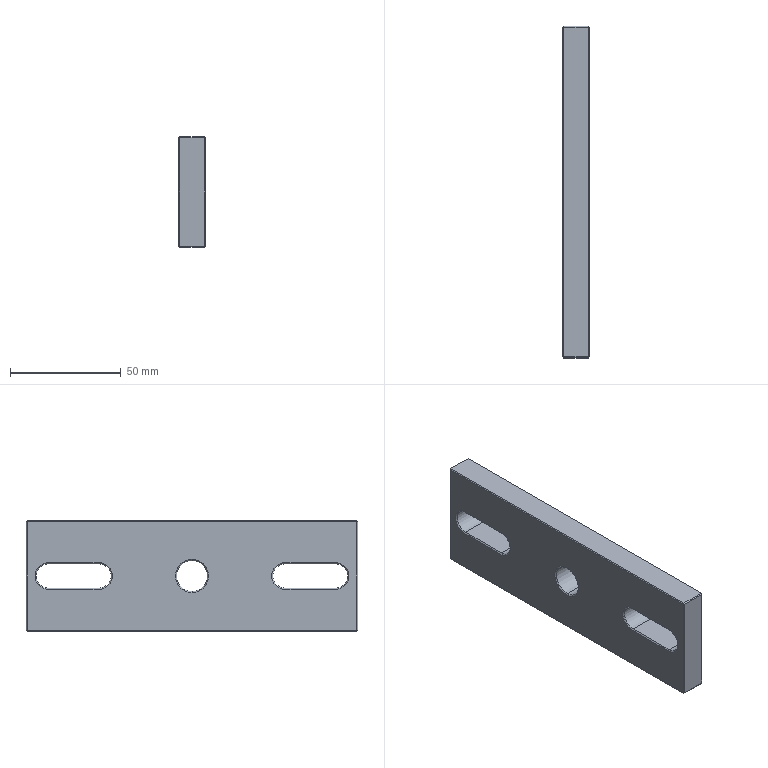Part | SolidWorks | features BaseBody 1 | 1 solid | 56 faces | box 12 x 150 x 50 mm | volume 79643 mm3 | plane 38 | cone 12 | cylinder 6 | commonest cylinder face diameters 11 x4 14 x2
STEP:
#1=CARTESIAN_POINT('',(-36.5,279.,-7.));
#2=VERTEX_POINT('',#1);
#3=CARTESIAN_POINT('',(-36.5,279.,7.));
#4=VERTEX_POINT('',#3);
#5=CARTESIAN_POINT('',(-36.5,279.,0.));
#6=DIRECTION('',(-1.,0.,0.));
#7=DIRECTION('',(0.,0.,1.));
#8=AXIS2_PLACEMENT_3D('',#5,#6,#7);
#9=CIRCLE('',#8,7.);
#10=EDGE_CURVE('',#2,#4,#9,.T.);
#11=ORIENTED_EDGE('',*,*,#10,.F.);
#12=CARTESIAN_POINT('',(-37.,279.,-7.5));
#13=VERTEX_POINT('',#12);
#14=CARTESIAN_POINT('',(-37.,279.,-7.5));
#15=DIRECTION('',(-0.7071,0.,-0.7071));
#16=VECTOR('',#15,1000.);
#17=LINE('',#14,#16);
#18=EDGE_CURVE('',#2,#13,#17,.T.);
#19=ORIENTED_EDGE('',*,*,#18,.T.);
#20=CARTESIAN_POINT('',(-37.,279.,7.5));
#21=VERTEX_POINT('',#20);
#22=CARTESIAN_POINT('',(-37.,279.,0.));
#23=DIRECTION('',(1.,0.,0.));
#24=DIRECTION('',(0.,0.,1.));
#25=AXIS2_PLACEMENT_3D('',#22,#23,#24);
#26=CIRCLE('',#25,7.5);
#27=EDGE_CURVE('',#21,#13,#26,.T.);
#28=ORIENTED_EDGE('',*,*,#27,.F.);
#29=CARTESIAN_POINT('',(-37.,279.,7.5));
#30=DIRECTION('',(-0.7071,0.,0.7071));
#31=VECTOR('',#30,1000.);
#32=LINE('',#29,#31);
#33=EDGE_CURVE('',#4,#21,#32,.T.);
#34=ORIENTED_EDGE('',*,*,#33,.F.);
#35=EDGE_LOOP('',(#11,#19,#28,#34));
#36=FACE_OUTER_BOUND('',#35,.T.);
#37=CARTESIAN_POINT('',(-37.,279.,0.));
#38=DIRECTION('',(-1.,0.,0.));
#39=DIRECTION('',(0.,0.,1.));
#40=AXIS2_PLACEMENT_3D('',#37,#38,#39);
#41=CONICAL_SURFACE('',#40,7.5,0.7854);
#42=ADVANCED_FACE('',(#36),#41,.F.);
#43=CARTESIAN_POINT('',(-25.5,279.,7.));
#44=VERTEX_POINT('',#43);
#45=CARTESIAN_POINT('',(-25.5,279.,-7.));
#46=VERTEX_POINT('',#45);
#47=CARTESIAN_POINT('',(-25.5,279.,0.));
#48=DIRECTION('',(1.,0.,0.));
#49=DIRECTION('',(0.,0.,1.));
#50=AXIS2_PLACEMENT_3D('',#47,#48,#49);
#51=CIRCLE('',#50,7.);
#52=EDGE_CURVE('',#44,#46,#51,.T.);
#53=ORIENTED_EDGE('',*,*,#52,.F.);
#54=CARTESIAN_POINT('',(-25.,279.,7.5));
#55=VERTEX_POINT('',#54);
#56=CARTESIAN_POINT('',(-25.5,279.,7.));
#57=DIRECTION('',(0.7071,0.,0.7071));
#58=VECTOR('',#57,1000.);
#59=LINE('',#56,#58);
#60=EDGE_CURVE('',#44,#55,#59,.T.);
#61=ORIENTED_EDGE('',*,*,#60,.T.);
#62=CARTESIAN_POINT('',(-25.,279.,-7.5));
#63=VERTEX_POINT('',#62);
#64=CARTESIAN_POINT('',(-25.,279.,0.));
#65=DIRECTION('',(-1.,0.,0.));
#66=DIRECTION('',(0.,0.,1.));
#67=AXIS2_PLACEMENT_3D('',#64,#65,#66);
#68=CIRCLE('',#67,7.5);
#69=EDGE_CURVE('',#63,#55,#68,.T.);
#70=ORIENTED_EDGE('',*,*,#69,.F.);
#71=CARTESIAN_POINT('',(-25.5,279.,-7.));
#72=DIRECTION('',(0.7071,0.,-0.7071));
#73=VECTOR('',#72,1000.);
#74=LINE('',#71,#73);
#75=EDGE_CURVE('',#46,#63,#74,.T.);
#76=ORIENTED_EDGE('',*,*,#75,.F.);
#77=EDGE_LOOP('',(#53,#61,#70,#76));
#78=FACE_OUTER_BOUND('',#77,.T.);
#79=CARTESIAN_POINT('',(-25.5,279.,0.));
#80=DIRECTION('',(1.,0.,0.));
#81=DIRECTION('',(0.,0.,-1.));
#82=AXIS2_PLACEMENT_3D('',#79,#80,#81);
#83=CONICAL_SURFACE('',#82,7.,0.7854);
#84=ADVANCED_FACE('',(#78),#83,.F.);
#85=ORIENTED_EDGE('',*,*,#10,.T.);
#86=CARTESIAN_POINT('',(-25.,279.,7.));
#87=DIRECTION('',(1.,0.,0.));
#88=VECTOR('',#87,1000.);
#89=LINE('',#86,#88);
#90=EDGE_CURVE('',#4,#44,#89,.T.);
#91=ORIENTED_EDGE('',*,*,#90,.T.);
#92=ORIENTED_EDGE('',*,*,#52,.T.);
#93=CARTESIAN_POINT('',(-25.,279.,-7.));
#94=DIRECTION('',(1.,0.,0.));
#95=VECTOR('',#94,1000.);
#96=LINE('',#93,#95);
#97=EDGE_CURVE('',#2,#46,#96,.T.);
#98=ORIENTED_EDGE('',*,*,#97,.F.);
#99=EDGE_LOOP('',(#85,#91,#92,#98));
#100=FACE_OUTER_BOUND('',#99,.T.);
#101=CARTESIAN_POINT('',(-25.,279.,0.));
#102=DIRECTION('',(1.,0.,0.));
#103=DIRECTION('',(0.,0.,-1.));
#104=AXIS2_PLACEMENT_3D('',#101,#102,#103);
#105=CYLINDRICAL_SURFACE('',#104,7.);
#106=ADVANCED_FACE('',(#100),#105,.F.);
#107=CARTESIAN_POINT('',(-36.5,214.,-5.5));
#108=VERTEX_POINT('',#107);
#109=CARTESIAN_POINT('',(-37.,214.,-6.));
#110=VERTEX_POINT('',#109);
#111=CARTESIAN_POINT('',(-36.5,214.,-5.5));
#112=DIRECTION('',(-0.7071,0.,-0.7071));
#113=VECTOR('',#112,1000.);
#114=LINE('',#111,#113);
#115=EDGE_CURVE('',#108,#110,#114,.T.);
#116=ORIENTED_EDGE('',*,*,#115,.T.);
#117=CARTESIAN_POINT('',(-37.,214.,6.));
#118=VERTEX_POINT('',#117);
#119=CARTESIAN_POINT('',(-37.,214.,0.));
#120=DIRECTION('',(1.,0.,0.));
#121=DIRECTION('',(0.,0.,1.));
#122=AXIS2_PLACEMENT_3D('',#119,#120,#121);
#123=CIRCLE('',#122,6.);
#124=EDGE_CURVE('',#118,#110,#123,.T.);
#125=ORIENTED_EDGE('',*,*,#124,.F.);
#126=CARTESIAN_POINT('',(-36.5,214.,5.5));
#127=VERTEX_POINT('',#126);
#128=CARTESIAN_POINT('',(-37.,214.,6.));
#129=DIRECTION('',(0.7071,0.,-0.7071));
#130=VECTOR('',#129,1000.);
#131=LINE('',#128,#130);
#132=EDGE_CURVE('',#118,#127,#131,.T.);
#133=ORIENTED_EDGE('',*,*,#132,.T.);
#134=CARTESIAN_POINT('',(-36.5,214.,0.));
#135=DIRECTION('',(-1.,0.,0.));
#136=DIRECTION('',(0.,0.,1.));
#137=AXIS2_PLACEMENT_3D('',#134,#135,#136);
#138=CIRCLE('',#137,5.5);
#139=EDGE_CURVE('',#108,#127,#138,.T.);
#140=ORIENTED_EDGE('',*,*,#139,.F.);
#141=EDGE_LOOP('',(#116,#125,#133,#140));
#142=FACE_OUTER_BOUND('',#141,.T.);
#143=CARTESIAN_POINT('',(-36.5,214.,0.));
#144=DIRECTION('',(-1.,0.,0.));
#145=DIRECTION('',(0.,0.,1.));
#146=AXIS2_PLACEMENT_3D('',#143,#144,#145);
#147=CONICAL_SURFACE('',#146,5.5,0.7854);
#148=ADVANCED_FACE('',(#142),#147,.F.);
#149=CARTESIAN_POINT('',(-37.,237.,6.));
#150=VERTEX_POINT('',#149);
#151=CARTESIAN_POINT('',(-36.5,237.,5.5));
#152=VERTEX_POINT('',#151);
#153=CARTESIAN_POINT('',(-37.,237.,6.));
#154=DIRECTION('',(0.7071,0.,-0.7071));
#155=VECTOR('',#154,1000.);
#156=LINE('',#153,#155);
#157=EDGE_CURVE('',#150,#152,#156,.T.);
#158=ORIENTED_EDGE('',*,*,#157,.T.);
#159=CARTESIAN_POINT('',(-36.5,237.,5.5));
#160=DIRECTION('',(0.,1.,0.));
#161=VECTOR('',#160,1000.);
#162=LINE('',#159,#161);
#163=EDGE_CURVE('',#127,#152,#162,.T.);
#164=ORIENTED_EDGE('',*,*,#163,.F.);
#165=ORIENTED_EDGE('',*,*,#132,.F.);
#166=CARTESIAN_POINT('',(-37.,214.,6.));
#167=DIRECTION('',(0.,-1.,0.));
#168=VECTOR('',#167,1000.);
#169=LINE('',#166,#168);
#170=EDGE_CURVE('',#150,#118,#169,.T.);
#171=ORIENTED_EDGE('',*,*,#170,.F.);
#172=EDGE_LOOP('',(#158,#164,#165,#171));
#173=FACE_OUTER_BOUND('',#172,.T.);
#174=CARTESIAN_POINT('',(-36.5,247.,5.5));
#175=DIRECTION('',(-0.7071,0.,-0.7071));
#176=DIRECTION('',(-0.7071,0.,0.7071));
#177=AXIS2_PLACEMENT_3D('',#174,#175,#176);
#178=PLANE('',#177);
#179=ADVANCED_FACE('',(#173),#178,.T.);
#180=CARTESIAN_POINT('',(-36.5,237.,-5.5));
#181=VERTEX_POINT('',#180);
#182=CARTESIAN_POINT('',(-37.,237.,-6.));
#183=VERTEX_POINT('',#182);
#184=CARTESIAN_POINT('',(-36.5,237.,-5.5));
#185=DIRECTION('',(-0.7071,0.,-0.7071));
#186=VECTOR('',#185,1000.);
#187=LINE('',#184,#186);
#188=EDGE_CURVE('',#181,#183,#187,.T.);
#189=ORIENTED_EDGE('',*,*,#188,.T.);
#190=CARTESIAN_POINT('',(-37.,237.,-6.));
#191=DIRECTION('',(0.,1.,0.));
#192=VECTOR('',#191,1000.);
#193=LINE('',#190,#192);
#194=EDGE_CURVE('',#110,#183,#193,.T.);
#195=ORIENTED_EDGE('',*,*,#194,.F.);
#196=ORIENTED_EDGE('',*,*,#115,.F.);
#197=CARTESIAN_POINT('',(-36.5,214.,-5.5));
#198=DIRECTION('',(0.,-1.,0.));
#199=VECTOR('',#198,1000.);
#200=LINE('',#197,#199);
#201=EDGE_CURVE('',#181,#108,#200,.T.);
#202=ORIENTED_EDGE('',*,*,#201,.F.);
#203=EDGE_LOOP('',(#189,#195,#196,#202));
#204=FACE_OUTER_BOUND('',#203,.T.);
#205=CARTESIAN_POINT('',(-36.5,247.,-5.5));
#206=DIRECTION('',(-0.7071,0.,0.7071));
#207=DIRECTION('',(0.,1.,0.));
#208=AXIS2_PLACEMENT_3D('',#205,#206,#207);
#209=PLANE('',#208);
#210=ADVANCED_FACE('',(#204),#209,.T.);
#211=ORIENTED_EDGE('',*,*,#157,.F.);
#212=CARTESIAN_POINT('',(-37.,237.,0.));
#213=DIRECTION('',(1.,0.,0.));
#214=DIRECTION('',(0.,0.,1.));
#215=AXIS2_PLACEMENT_3D('',#212,#213,#214);
#216=CIRCLE('',#215,6.);
#217=EDGE_CURVE('',#183,#150,#216,.T.);
#218=ORIENTED_EDGE('',*,*,#217,.F.);
#219=ORIENTED_EDGE('',*,*,#188,.F.);
#220=CARTESIAN_POINT('',(-36.5,237.,0.));
#221=DIRECTION('',(-1.,0.,0.));
#222=DIRECTION('',(0.,0.,1.));
#223=AXIS2_PLACEMENT_3D('',#220,#221,#222);
#224=CIRCLE('',#223,5.5);
#225=EDGE_CURVE('',#152,#181,#224,.T.);
#226=ORIENTED_EDGE('',*,*,#225,.F.);
#227=EDGE_LOOP('',(#211,#218,#219,#226));
#228=FACE_OUTER_BOUND('',#227,.T.);
#229=CARTESIAN_POINT('',(-36.5,237.,0.));
#230=DIRECTION('',(-1.,0.,0.));
#231=DIRECTION('',(0.,0.,1.));
#232=AXIS2_PLACEMENT_3D('',#229,#230,#231);
#233=CONICAL_SURFACE('',#232,5.5,0.7854);
#234=ADVANCED_FACE('',(#228),#233,.F.);
#235=CARTESIAN_POINT('',(-25.5,237.,-5.5));
#236=VERTEX_POINT('',#235);
#237=CARTESIAN_POINT('',(-25.,237.,-6.));
#238=VERTEX_POINT('',#237);
#239=CARTESIAN_POINT('',(-25.5,237.,-5.5));
#240=DIRECTION('',(0.7071,0.,-0.7071));
#241=VECTOR('',#240,1000.);
#242=LINE('',#239,#241);
#243=EDGE_CURVE('',#236,#238,#242,.T.);
#244=ORIENTED_EDGE('',*,*,#243,.T.);
#245=CARTESIAN_POINT('',(-25.,237.,6.));
#246=VERTEX_POINT('',#245);
#247=CARTESIAN_POINT('',(-25.,237.,0.));
#248=DIRECTION('',(-1.,0.,0.));
#249=DIRECTION('',(0.,0.,1.));
#250=AXIS2_PLACEMENT_3D('',#247,#248,#249);
#251=CIRCLE('',#250,6.);
#252=EDGE_CURVE('',#246,#238,#251,.T.);
#253=ORIENTED_EDGE('',*,*,#252,.F.);
#254=CARTESIAN_POINT('',(-25.5,237.,5.5));
#255=VERTEX_POINT('',#254);
#256=CARTESIAN_POINT('',(-25.,237.,6.));
#257=DIRECTION('',(-0.7071,0.,-0.7071));
#258=VECTOR('',#257,1000.);
#259=LINE('',#256,#258);
#260=EDGE_CURVE('',#246,#255,#259,.T.);
#261=ORIENTED_EDGE('',*,*,#260,.T.);
#262=CARTESIAN_POINT('',(-25.5,237.,0.));
#263=DIRECTION('',(1.,0.,0.));
#264=DIRECTION('',(0.,0.,1.));
#265=AXIS2_PLACEMENT_3D('',#262,#263,#264);
#266=CIRCLE('',#265,5.5);
#267=EDGE_CURVE('',#236,#255,#266,.T.);
#268=ORIENTED_EDGE('',*,*,#267,.F.);
#269=EDGE_LOOP('',(#244,#253,#261,#268));
#270=FACE_OUTER_BOUND('',#269,.T.);
#271=CARTESIAN_POINT('',(-25.5,237.,0.));
#272=DIRECTION('',(1.,0.,0.));
#273=DIRECTION('',(0.,0.,-1.));
#274=AXIS2_PLACEMENT_3D('',#271,#272,#273);
#275=CONICAL_SURFACE('',#274,5.5,0.7854);
#276=ADVANCED_FACE('',(#270),#275,.F.);
#277=CARTESIAN_POINT('',(-25.,214.,6.));
#278=VERTEX_POINT('',#277);
#279=CARTESIAN_POINT('',(-25.5,214.,5.5));
#280=VERTEX_POINT('',#279);
#281=CARTESIAN_POINT('',(-25.,214.,6.));
#282=DIRECTION('',(-0.7071,0.,-0.7071));
#283=VECTOR('',#282,1000.);
#284=LINE('',#281,#283);
#285=EDGE_CURVE('',#278,#280,#284,.T.);
#286=ORIENTED_EDGE('',*,*,#285,.T.);
#287=CARTESIAN_POINT('',(-25.5,247.,5.5));
#288=DIRECTION('',(0.,-1.,0.));
#289=VECTOR('',#288,1000.);
#290=LINE('',#287,#289);
#291=EDGE_CURVE('',#255,#280,#290,.T.);
#292=ORIENTED_EDGE('',*,*,#291,.F.);
#293=ORIENTED_EDGE('',*,*,#260,.F.);
#294=CARTESIAN_POINT('',(-25.,533.,6.));
#295=DIRECTION('',(0.,1.,0.));
#296=VECTOR('',#295,1000.);
#297=LINE('',#294,#296);
#298=EDGE_CURVE('',#278,#246,#297,.T.);
#299=ORIENTED_EDGE('',*,*,#298,.F.);
#300=EDGE_LOOP('',(#286,#292,#293,#299));
#301=FACE_OUTER_BOUND('',#300,.T.);
#302=CARTESIAN_POINT('',(-25.5,247.,5.5));
#303=DIRECTION('',(-0.7071,0.,0.7071));
#304=DIRECTION('',(0.,1.,0.));
#305=AXIS2_PLACEMENT_3D('',#302,#303,#304);
#306=PLANE('',#305);
#307=ADVANCED_FACE('',(#301),#306,.F.);
#308=CARTESIAN_POINT('',(-25.5,214.,-5.5));
#309=VERTEX_POINT('',#308);
#310=CARTESIAN_POINT('',(-25.,214.,-6.));
#311=VERTEX_POINT('',#310);
#312=CARTESIAN_POINT('',(-25.5,214.,-5.5));
#313=DIRECTION('',(0.7071,0.,-0.7071));
#314=VECTOR('',#313,1000.);
#315=LINE('',#312,#314);
#316=EDGE_CURVE('',#309,#311,#315,.T.);
#317=ORIENTED_EDGE('',*,*,#316,.T.);
#318=CARTESIAN_POINT('',(-25.,533.,-6.));
#319=DIRECTION('',(0.,-1.,0.));
#320=VECTOR('',#319,1000.);
#321=LINE('',#318,#320);
#322=EDGE_CURVE('',#238,#311,#321,.T.);
#323=ORIENTED_EDGE('',*,*,#322,.F.);
#324=ORIENTED_EDGE('',*,*,#243,.F.);
#325=CARTESIAN_POINT('',(-25.5,247.,-5.5));
#326=DIRECTION('',(0.,1.,0.));
#327=VECTOR('',#326,1000.);
#328=LINE('',#325,#327);
#329=EDGE_CURVE('',#309,#236,#328,.T.);
#330=ORIENTED_EDGE('',*,*,#329,.F.);
#331=EDGE_LOOP('',(#317,#323,#324,#330));
#332=FACE_OUTER_BOUND('',#331,.T.);
#333=CARTESIAN_POINT('',(-25.,533.,-6.));
#334=DIRECTION('',(-0.7071,0.,-0.7071));
#335=DIRECTION('',(-0.7071,0.,0.7071));
#336=AXIS2_PLACEMENT_3D('',#333,#334,#335);
#337=PLANE('',#336);
#338=ADVANCED_FACE('',(#332),#337,.F.);
#339=ORIENTED_EDGE('',*,*,#285,.F.);
#340=CARTESIAN_POINT('',(-25.,214.,0.));
#341=DIRECTION('',(-1.,0.,0.));
#342=DIRECTION('',(0.,0.,1.));
#343=AXIS2_PLACEMENT_3D('',#340,#341,#342);
#344=CIRCLE('',#343,6.);
#345=EDGE_CURVE('',#311,#278,#344,.T.);
#346=ORIENTED_EDGE('',*,*,#345,.F.);
#347=ORIENTED_EDGE('',*,*,#316,.F.);
#348=CARTESIAN_POINT('',(-25.5,214.,0.));
#349=DIRECTION('',(1.,0.,0.));
#350=DIRECTION('',(0.,0.,1.));
#351=AXIS2_PLACEMENT_3D('',#348,#349,#350);
#352=CIRCLE('',#351,5.5);
#353=EDGE_CURVE('',#280,#309,#352,.T.);
#354=ORIENTED_EDGE('',*,*,#353,.F.);
#355=EDGE_LOOP('',(#339,#346,#347,#354));
#356=FACE_OUTER_BOUND('',#355,.T.);
#357=CARTESIAN_POINT('',(-25.5,214.,0.));
#358=DIRECTION('',(1.,0.,0.));
#359=DIRECTION('',(0.,0.,-1.));
#360=AXIS2_PLACEMENT_3D('',#357,#358,#359);
#361=CONICAL_SURFACE('',#360,5.5,0.7854);
#362=ADVANCED_FACE('',(#356),#361,.F.);
#363=CARTESIAN_POINT('',(-36.5,321.,5.5));
#364=VERTEX_POINT('',#363);
#365=CARTESIAN_POINT('',(-37.,321.,6.));
#366=VERTEX_POINT('',#365);
#367=CARTESIAN_POINT('',(-36.5,321.,5.5));
#368=DIRECTION('',(-0.7071,0.,0.7071));
#369=VECTOR('',#368,1000.);
#370=LINE('',#367,#369);
#371=EDGE_CURVE('',#364,#366,#370,.T.);
#372=ORIENTED_EDGE('',*,*,#371,.T.);
#373=CARTESIAN_POINT('',(-37.,344.,6.));
#374=VERTEX_POINT('',#373);
#375=CARTESIAN_POINT('',(-37.,321.,6.));
#376=DIRECTION('',(0.,-1.,0.));
#377=VECTOR('',#376,1000.);
#378=LINE('',#375,#377);
#379=EDGE_CURVE('',#374,#366,#378,.T.);
#380=ORIENTED_EDGE('',*,*,#379,.F.);
#381=CARTESIAN_POINT('',(-36.5,344.,5.5));
#382=VERTEX_POINT('',#381);
#383=CARTESIAN_POINT('',(-37.,344.,6.));
#384=DIRECTION('',(0.7071,0.,-0.7071));
#385=VECTOR('',#384,1000.);
#386=LINE('',#383,#385);
#387=EDGE_CURVE('',#374,#382,#386,.T.);
#388=ORIENTED_EDGE('',*,*,#387,.T.);
#389=CARTESIAN_POINT('',(-36.5,344.,5.5));
#390=DIRECTION('',(0.,1.,0.));
#391=VECTOR('',#390,1000.);
#392=LINE('',#389,#391);
#393=EDGE_CURVE('',#364,#382,#392,.T.);
#394=ORIENTED_EDGE('',*,*,#393,.F.);
#395=EDGE_LOOP('',(#372,#380,#388,#394));
#396=FACE_OUTER_BOUND('',#395,.T.);
#397=CARTESIAN_POINT('',(-36.5,347.,5.5));
#398=DIRECTION('',(-0.7071,0.,-0.7071));
#399=DIRECTION('',(-0.7071,0.,0.7071));
#400=AXIS2_PLACEMENT_3D('',#397,#398,#399);
#401=PLANE('',#400);
#402=ADVANCED_FACE('',(#396),#401,.T.);
#403=CARTESIAN_POINT('',(-37.,344.,-6.));
#404=VERTEX_POINT('',#403);
#405=CARTESIAN_POINT('',(-36.5,344.,-5.5));
#406=VERTEX_POINT('',#405);
#407=CARTESIAN_POINT('',(-37.,344.,-6.));
#408=DIRECTION('',(0.7071,0.,0.7071));
#409=VECTOR('',#408,1000.);
#410=LINE('',#407,#409);
#411=EDGE_CURVE('',#404,#406,#410,.T.);
#412=ORIENTED_EDGE('',*,*,#411,.T.);
#413=CARTESIAN_POINT('',(-36.5,344.,0.));
#414=DIRECTION('',(-1.,0.,0.));
#415=DIRECTION('',(0.,0.,1.));
#416=AXIS2_PLACEMENT_3D('',#413,#414,#415);
#417=CIRCLE('',#416,5.5);
#418=EDGE_CURVE('',#382,#406,#417,.T.);
#419=ORIENTED_EDGE('',*,*,#418,.F.);
#420=ORIENTED_EDGE('',*,*,#387,.F.);
#421=CARTESIAN_POINT('',(-37.,344.,0.));
#422=DIRECTION('',(1.,0.,0.));
#423=DIRECTION('',(0.,0.,1.));
#424=AXIS2_PLACEMENT_3D('',#421,#422,#423);
#425=CIRCLE('',#424,6.);
#426=EDGE_CURVE('',#404,#374,#425,.T.);
#427=ORIENTED_EDGE('',*,*,#426,.F.);
#428=EDGE_LOOP('',(#412,#419,#420,#427));
#429=FACE_OUTER_BOUND('',#428,.T.);
#430=CARTESIAN_POINT('',(-36.5,344.,0.));
#431=DIRECTION('',(-1.,0.,0.));
#432=DIRECTION('',(0.,0.,1.));
#433=AXIS2_PLACEMENT_3D('',#430,#431,#432);
#434=CONICAL_SURFACE('',#433,5.5,0.7854);
#435=ADVANCED_FACE('',(#429),#434,.F.);
#436=CARTESIAN_POINT('',(-36.5,321.,-5.5));
#437=VERTEX_POINT('',#436);
#438=CARTESIAN_POINT('',(-37.,321.,-6.));
#439=VERTEX_POINT('',#438);
#440=CARTESIAN_POINT('',(-36.5,321.,-5.5));
#441=DIRECTION('',(-0.7071,0.,-0.7071));
#442=VECTOR('',#441,1000.);
#443=LINE('',#440,#442);
#444=EDGE_CURVE('',#437,#439,#443,.T.);
#445=ORIENTED_EDGE('',*,*,#444,.T.);
#446=CARTESIAN_POINT('',(-37.,321.,0.));
#447=DIRECTION('',(1.,0.,0.));
#448=DIRECTION('',(0.,0.,1.));
#449=AXIS2_PLACEMENT_3D('',#446,#447,#448);
#450=CIRCLE('',#449,6.);
#451=EDGE_CURVE('',#366,#439,#450,.T.);
#452=ORIENTED_EDGE('',*,*,#451,.F.);
#453=ORIENTED_EDGE('',*,*,#371,.F.);
#454=CARTESIAN_POINT('',(-36.5,321.,0.));
#455=DIRECTION('',(-1.,0.,0.));
#456=DIRECTION('',(0.,0.,1.));
#457=AXIS2_PLACEMENT_3D('',#454,#455,#456);
#458=CIRCLE('',#457,5.5);
#459=EDGE_CURVE('',#437,#364,#458,.T.);
#460=ORIENTED_EDGE('',*,*,#459,.F.);
#461=EDGE_LOOP('',(#445,#452,#453,#460));
#462=FACE_OUTER_BOUND('',#461,.T.);
#463=CARTESIAN_POINT('',(-36.5,321.,0.));
#464=DIRECTION('',(-1.,0.,0.));
#465=DIRECTION('',(0.,0.,1.));
#466=AXIS2_PLACEMENT_3D('',#463,#464,#465);
#467=CONICAL_SURFACE('',#466,5.5,0.7854);
#468=ADVANCED_FACE('',(#462),#467,.F.);
#469=ORIENTED_EDGE('',*,*,#411,.F.);
#470=CARTESIAN_POINT('',(-37.,344.,-6.));
#471=DIRECTION('',(0.,1.,0.));
#472=VECTOR('',#471,1000.);
#473=LINE('',#470,#472);
#474=EDGE_CURVE('',#439,#404,#473,.T.);
#475=ORIENTED_EDGE('',*,*,#474,.F.);
#476=ORIENTED_EDGE('',*,*,#444,.F.);
#477=CARTESIAN_POINT('',(-36.5,321.,-5.5));
#478=DIRECTION('',(0.,-1.,0.));
#479=VECTOR('',#478,1000.);
#480=LINE('',#477,#479);
#481=EDGE_CURVE('',#406,#437,#480,.T.);
#482=ORIENTED_EDGE('',*,*,#481,.F.);
#483=EDGE_LOOP('',(#469,#475,#476,#482));
#484=FACE_OUTER_BOUND('',#483,.T.);
#485=CARTESIAN_POINT('',(-36.5,347.,-5.5));
#486=DIRECTION('',(-0.7071,0.,0.7071));
#487=DIRECTION('',(0.,1.,0.));
#488=AXIS2_PLACEMENT_3D('',#485,#486,#487);
#489=PLANE('',#488);
#490=ADVANCED_FACE('',(#484),#489,.T.);
#491=CARTESIAN_POINT('',(-25.5,344.,-5.5));
#492=VERTEX_POINT('',#491);
#493=CARTESIAN_POINT('',(-25.,344.,-6.));
#494=VERTEX_POINT('',#493);
#495=CARTESIAN_POINT('',(-25.5,344.,-5.5));
#496=DIRECTION('',(0.7071,0.,-0.7071));
#497=VECTOR('',#496,1000.);
#498=LINE('',#495,#497);
#499=EDGE_CURVE('',#492,#494,#498,.T.);
#500=ORIENTED_EDGE('',*,*,#499,.T.);
#501=CARTESIAN_POINT('',(-25.,344.,6.));
#502=VERTEX_POINT('',#501);
#503=CARTESIAN_POINT('',(-25.,344.,0.));
#504=DIRECTION('',(-1.,0.,0.));
#505=DIRECTION('',(0.,0.,1.));
#506=AXIS2_PLACEMENT_3D('',#503,#504,#505);
#507=CIRCLE('',#506,6.);
#508=EDGE_CURVE('',#502,#494,#507,.T.);
#509=ORIENTED_EDGE('',*,*,#508,.F.);
#510=CARTESIAN_POINT('',(-25.5,344.,5.5));
#511=VERTEX_POINT('',#510);
#512=CARTESIAN_POINT('',(-25.,344.,6.));
#513=DIRECTION('',(-0.7071,0.,-0.7071));
#514=VECTOR('',#513,1000.);
#515=LINE('',#512,#514);
#516=EDGE_CURVE('',#502,#511,#515,.T.);
#517=ORIENTED_EDGE('',*,*,#516,.T.);
#518=CARTESIAN_POINT('',(-25.5,344.,0.));
#519=DIRECTION('',(1.,0.,0.));
#520=DIRECTION('',(0.,0.,1.));
#521=AXIS2_PLACEMENT_3D('',#518,#519,#520);
#522=CIRCLE('',#521,5.5);
#523=EDGE_CURVE('',#492,#511,#522,.T.);
#524=ORIENTED_EDGE('',*,*,#523,.F.);
#525=EDGE_LOOP('',(#500,#509,#517,#524));
#526=FACE_OUTER_BOUND('',#525,.T.);
#527=CARTESIAN_POINT('',(-25.5,344.,0.));
#528=DIRECTION('',(1.,0.,0.));
#529=DIRECTION('',(0.,0.,-1.));
#530=AXIS2_PLACEMENT_3D('',#527,#528,#529);
#531=CONICAL_SURFACE('',#530,5.5,0.7854);
#532=ADVANCED_FACE('',(#526),#531,.F.);
#533=CARTESIAN_POINT('',(-25.,321.,6.));
#534=VERTEX_POINT('',#533);
#535=CARTESIAN_POINT('',(-25.5,321.,5.5));
#536=VERTEX_POINT('',#535);
#537=CARTESIAN_POINT('',(-25.,321.,6.));
#538=DIRECTION('',(-0.7071,0.,-0.7071));
#539=VECTOR('',#538,1000.);
#540=LINE('',#537,#539);
#541=EDGE_CURVE('',#534,#536,#540,.T.);
#542=ORIENTED_EDGE('',*,*,#541,.T.);
#543=CARTESIAN_POINT('',(-25.5,347.,5.5));
#544=DIRECTION('',(0.,-1.,0.));
#545=VECTOR('',#544,1000.);
#546=LINE('',#543,#545);
#547=EDGE_CURVE('',#511,#536,#546,.T.);
#548=ORIENTED_EDGE('',*,*,#547,.F.);
#549=ORIENTED_EDGE('',*,*,#516,.F.);
#550=CARTESIAN_POINT('',(-25.,533.,6.));
#551=DIRECTION('',(0.,1.,0.));
#552=VECTOR('',#551,1000.);
#553=LINE('',#550,#552);
#554=EDGE_CURVE('',#534,#502,#553,.T.);
#555=ORIENTED_EDGE('',*,*,#554,.F.);
#556=EDGE_LOOP('',(#542,#548,#549,#555));
#557=FACE_OUTER_BOUND('',#556,.T.);
#558=CARTESIAN_POINT('',(-25.5,347.,5.5));
#559=DIRECTION('',(-0.7071,0.,0.7071));
#560=DIRECTION('',(0.,1.,0.));
#561=AXIS2_PLACEMENT_3D('',#558,#559,#560);
#562=PLANE('',#561);
#563=ADVANCED_FACE('',(#557),#562,.F.);
#564=CARTESIAN_POINT('',(-25.5,321.,-5.5));
#565=VERTEX_POINT('',#564);
#566=CARTESIAN_POINT('',(-25.,321.,-6.));
#567=VERTEX_POINT('',#566);
#568=CARTESIAN_POINT('',(-25.5,321.,-5.5));
#569=DIRECTION('',(0.7071,0.,-0.7071));
#570=VECTOR('',#569,1000.);
#571=LINE('',#568,#570);
#572=EDGE_CURVE('',#565,#567,#571,.T.);
#573=ORIENTED_EDGE('',*,*,#572,.T.);
#574=CARTESIAN_POINT('',(-25.,533.,-6.));
#575=DIRECTION('',(0.,-1.,0.));
#576=VECTOR('',#575,1000.);
#577=LINE('',#574,#576);
#578=EDGE_CURVE('',#494,#567,#577,.T.);
#579=ORIENTED_EDGE('',*,*,#578,.F.);
#580=ORIENTED_EDGE('',*,*,#499,.F.);
#581=CARTESIAN_POINT('',(-25.5,347.,-5.5));
#582=DIRECTION('',(0.,1.,0.));
#583=VECTOR('',#582,1000.);
#584=LINE('',#581,#583);
#585=EDGE_CURVE('',#565,#492,#584,.T.);
#586=ORIENTED_EDGE('',*,*,#585,.F.);
#587=EDGE_LOOP('',(#573,#579,#580,#586));
#588=FACE_OUTER_BOUND('',#587,.T.);
#589=CARTESIAN_POINT('',(-25.,533.,-6.));
#590=DIRECTION('',(-0.7071,0.,-0.7071));
#591=DIRECTION('',(-0.7071,0.,0.7071));
#592=AXIS2_PLACEMENT_3D('',#589,#590,#591);
#593=PLANE('',#592);
#594=ADVANCED_FACE('',(#588),#593,.F.);
#595=ORIENTED_EDGE('',*,*,#541,.F.);
#596=CARTESIAN_POINT('',(-25.,321.,0.));
#597=DIRECTION('',(-1.,0.,0.));
#598=DIRECTION('',(0.,0.,1.));
#599=AXIS2_PLACEMENT_3D('',#596,#597,#598);
#600=CIRCLE('',#599,6.);
#601=EDGE_CURVE('',#567,#534,#600,.T.);
#602=ORIENTED_EDGE('',*,*,#601,.F.);
#603=ORIENTED_EDGE('',*,*,#572,.F.);
#604=CARTESIAN_POINT('',(-25.5,321.,0.));
#605=DIRECTION('',(1.,0.,0.));
#606=DIRECTION('',(0.,0.,1.));
#607=AXIS2_PLACEMENT_3D('',#604,#605,#606);
#608=CIRCLE('',#607,5.5);
#609=EDGE_CURVE('',#536,#565,#608,.T.);
#610=ORIENTED_EDGE('',*,*,#609,.F.);
#611=EDGE_LOOP('',(#595,#602,#603,#610));
#612=FACE_OUTER_BOUND('',#611,.T.);
#613=CARTESIAN_POINT('',(-25.5,321.,0.));
#614=DIRECTION('',(1.,0.,0.));
#615=DIRECTION('',(0.,0.,-1.));
#616=AXIS2_PLACEMENT_3D('',#613,#614,#615);
#617=CONICAL_SURFACE('',#616,5.5,0.7854);
#618=ADVANCED_FACE('',(#612),#617,.F.);
#619=CARTESIAN_POINT('',(-25.,204.5,-24.5));
#620=VERTEX_POINT('',#619);
#621=CARTESIAN_POINT('',(-25.5,204.5,-25.));
#622=VERTEX_POINT('',#621);
#623=CARTESIAN_POINT('',(-25.5,204.5,-25.));
#624=DIRECTION('',(-0.7071,0.,-0.7071));
#625=VECTOR('',#624,1000.);
#626=LINE('',#623,#625);
#627=EDGE_CURVE('',#620,#622,#626,.T.);
#628=ORIENTED_EDGE('',*,*,#627,.T.);
#629=CARTESIAN_POINT('',(-25.5,353.5,-25.));
#630=VERTEX_POINT('',#629);
#631=CARTESIAN_POINT('',(-25.5,204.,-25.));
#632=DIRECTION('',(0.,-1.,0.));
#633=VECTOR('',#632,1000.);
#634=LINE('',#631,#633);
#635=EDGE_CURVE('',#630,#622,#634,.T.);
#636=ORIENTED_EDGE('',*,*,#635,.F.);
#637=CARTESIAN_POINT('',(-25.,353.5,-24.5));
#638=VERTEX_POINT('',#637);
#639=CARTESIAN_POINT('',(-25.,353.5,-24.5));
#640=DIRECTION('',(0.7071,0.,0.7071));
#641=VECTOR('',#640,1000.);
#642=LINE('',#639,#641);
#643=EDGE_CURVE('',#630,#638,#642,.T.);
#644=ORIENTED_EDGE('',*,*,#643,.T.);
#645=CARTESIAN_POINT('',(-25.,533.,-24.5));
#646=DIRECTION('',(0.,1.,0.));
#647=VECTOR('',#646,1000.);
#648=LINE('',#645,#647);
#649=EDGE_CURVE('',#620,#638,#648,.T.);
#650=ORIENTED_EDGE('',*,*,#649,.F.);
#651=EDGE_LOOP('',(#628,#636,#644,#650));
#652=FACE_OUTER_BOUND('',#651,.T.);
#653=CARTESIAN_POINT('',(-25.,533.,-24.5));
#654=DIRECTION('',(-0.7071,0.,0.7071));
#655=DIRECTION('',(0.,1.,0.));
#656=AXIS2_PLACEMENT_3D('',#653,#654,#655);
#657=PLANE('',#656);
#658=ADVANCED_FACE('',(#652),#657,.F.);
#659=CARTESIAN_POINT('',(-25.5,354.,-24.5));
#660=VERTEX_POINT('',#659);
#661=CARTESIAN_POINT('',(-25.5,353.75,-24.75));
#662=DIRECTION('',(0.,0.7071,0.7071));
#663=VECTOR('',#662,1000.);
#664=LINE('',#661,#663);
#665=EDGE_CURVE('',#630,#660,#664,.T.);
#666=ORIENTED_EDGE('',*,*,#665,.T.);
#667=CARTESIAN_POINT('',(-25.,353.5,-24.5));
#668=DIRECTION('',(0.7071,-0.7071,0.));
#669=VECTOR('',#668,1000.);
#670=LINE('',#667,#669);
#671=EDGE_CURVE('',#660,#638,#670,.T.);
#672=ORIENTED_EDGE('',*,*,#671,.T.);
#673=ORIENTED_EDGE('',*,*,#643,.F.);
#674=EDGE_LOOP('',(#666,#672,#673));
#675=FACE_OUTER_BOUND('',#674,.T.);
#676=CARTESIAN_POINT('',(-25.,353.5,-24.5));
#677=DIRECTION('',(0.5774,0.5774,-0.5774));
#678=DIRECTION('',(0.,-0.7071,-0.7071));
#679=AXIS2_PLACEMENT_3D('',#676,#677,#678);
#680=PLANE('',#679);
#681=ADVANCED_FACE('',(#675),#680,.T.);
#682=CARTESIAN_POINT('',(-25.5,204.,-24.5));
#683=VERTEX_POINT('',#682);
#684=CARTESIAN_POINT('',(-25.25,204.25,-24.5));
#685=DIRECTION('',(-0.7071,-0.7071,0.));
#686=VECTOR('',#685,1000.);
#687=LINE('',#684,#686);
#688=EDGE_CURVE('',#620,#683,#687,.T.);
#689=ORIENTED_EDGE('',*,*,#688,.T.);
#690=CARTESIAN_POINT('',(-25.5,204.5,-25.));
#691=DIRECTION('',(0.,0.7071,-0.7071));
#692=VECTOR('',#691,1000.);
#693=LINE('',#690,#692);
#694=EDGE_CURVE('',#683,#622,#693,.T.);
#695=ORIENTED_EDGE('',*,*,#694,.T.);
#696=ORIENTED_EDGE('',*,*,#627,.F.);
#697=EDGE_LOOP('',(#689,#695,#696));
#698=FACE_OUTER_BOUND('',#697,.T.);
#699=CARTESIAN_POINT('',(-25.5,204.5,-25.));
#700=DIRECTION('',(0.5774,-0.5774,-0.5774));
#701=DIRECTION('',(0.,-0.7071,0.7071));
#702=AXIS2_PLACEMENT_3D('',#699,#700,#701);
#703=PLANE('',#702);
#704=ADVANCED_FACE('',(#698),#703,.T.);
#705=CARTESIAN_POINT('',(-36.5,353.5,-25.));
#706=VERTEX_POINT('',#705);
#707=CARTESIAN_POINT('',(-36.5,354.,-24.5));
#708=VERTEX_POINT('',#707);
#709=CARTESIAN_POINT('',(-36.5,353.5,-25.));
#710=DIRECTION('',(0.,0.7071,0.7071));
#711=VECTOR('',#710,1000.);
#712=LINE('',#709,#711);
#713=EDGE_CURVE('',#706,#708,#712,.T.);
#714=ORIENTED_EDGE('',*,*,#713,.T.);
#715=CARTESIAN_POINT('',(-37.,354.,-24.5));
#716=DIRECTION('',(-1.,0.,0.));
#717=VECTOR('',#716,1000.);
#718=LINE('',#715,#717);
#719=EDGE_CURVE('',#660,#708,#718,.T.);
#720=ORIENTED_EDGE('',*,*,#719,.F.);
#721=ORIENTED_EDGE('',*,*,#665,.F.);
#722=CARTESIAN_POINT('',(-37.,353.5,-25.));
#723=DIRECTION('',(1.,0.,0.));
#724=VECTOR('',#723,1000.);
#725=LINE('',#722,#724);
#726=EDGE_CURVE('',#706,#630,#725,.T.);
#727=ORIENTED_EDGE('',*,*,#726,.F.);
#728=EDGE_LOOP('',(#714,#720,#721,#727));
#729=FACE_OUTER_BOUND('',#728,.T.);
#730=CARTESIAN_POINT('',(-37.,353.5,-25.));
#731=DIRECTION('',(0.,-0.7071,0.7071));
#732=DIRECTION('',(-1.,0.,0.));
#733=AXIS2_PLACEMENT_3D('',#730,#731,#732);
#734=PLANE('',#733);
#735=ADVANCED_FACE('',(#729),#734,.F.);
#736=CARTESIAN_POINT('',(-25.5,354.,24.5));
#737=VERTEX_POINT('',#736);
#738=CARTESIAN_POINT('',(-25.,353.5,24.5));
#739=VERTEX_POINT('',#738);
#740=CARTESIAN_POINT('',(-25.,353.5,24.5));
#741=DIRECTION('',(0.7071,-0.7071,0.));
#742=VECTOR('',#741,1000.);
#743=LINE('',#740,#742);
#744=EDGE_CURVE('',#737,#739,#743,.T.);
#745=ORIENTED_EDGE('',*,*,#744,.T.);
#746=CARTESIAN_POINT('',(-25.,353.5,0.));
#747=DIRECTION('',(0.,0.,1.));
#748=VECTOR('',#747,1000.);
#749=LINE('',#746,#748);
#750=EDGE_CURVE('',#638,#739,#749,.T.);
#751=ORIENTED_EDGE('',*,*,#750,.F.);
#752=ORIENTED_EDGE('',*,*,#671,.F.);
#753=CARTESIAN_POINT('',(-25.5,354.,-25.));
#754=DIRECTION('',(0.,0.,-1.));
#755=VECTOR('',#754,1000.);
#756=LINE('',#753,#755);
#757=EDGE_CURVE('',#737,#660,#756,.T.);
#758=ORIENTED_EDGE('',*,*,#757,.F.);
#759=EDGE_LOOP('',(#745,#751,#752,#758));
#760=FACE_OUTER_BOUND('',#759,.T.);
#761=CARTESIAN_POINT('',(-25.,353.5,0.));
#762=DIRECTION('',(-0.7071,-0.7071,0.));
#763=DIRECTION('',(-0.7071,0.7071,0.));
#764=AXIS2_PLACEMENT_3D('',#761,#762,#763);
#765=PLANE('',#764);
#766=ADVANCED_FACE('',(#760),#765,.F.);
#767=CARTESIAN_POINT('',(-25.,204.5,24.5));
#768=VERTEX_POINT('',#767);
#769=CARTESIAN_POINT('',(-25.5,204.,24.5));
#770=VERTEX_POINT('',#769);
#771=CARTESIAN_POINT('',(-25.,204.5,24.5));
#772=DIRECTION('',(-0.7071,-0.7071,0.));
#773=VECTOR('',#772,1000.);
#774=LINE('',#771,#773);
#775=EDGE_CURVE('',#768,#770,#774,.T.);
#776=ORIENTED_EDGE('',*,*,#775,.T.);
#777=CARTESIAN_POINT('',(-25.5,204.,-25.));
#778=DIRECTION('',(0.,0.,1.));
#779=VECTOR('',#778,1000.);
#780=LINE('',#777,#779);
#781=EDGE_CURVE('',#683,#770,#780,.T.);
#782=ORIENTED_EDGE('',*,*,#781,.F.);
#783=ORIENTED_EDGE('',*,*,#688,.F.);
#784=CARTESIAN_POINT('',(-25.,204.5,0.));
#785=DIRECTION('',(0.,0.,-1.));
#786=VECTOR('',#785,1000.);
#787=LINE('',#784,#786);
#788=EDGE_CURVE('',#768,#620,#787,.T.);
#789=ORIENTED_EDGE('',*,*,#788,.F.);
#790=EDGE_LOOP('',(#776,#782,#783,#789));
#791=FACE_OUTER_BOUND('',#790,.T.);
#792=CARTESIAN_POINT('',(-25.,204.5,0.));
#793=DIRECTION('',(-0.7071,0.7071,0.));
#794=DIRECTION('',(0.,0.,1.));
#795=AXIS2_PLACEMENT_3D('',#792,#793,#794);
#796=PLANE('',#795);
#797=ADVANCED_FACE('',(#791),#796,.F.);
#798=CARTESIAN_POINT('',(-36.5,204.,-24.5));
#799=VERTEX_POINT('',#798);
#800=CARTESIAN_POINT('',(-36.5,204.5,-25.));
#801=VERTEX_POINT('',#800);
#802=CARTESIAN_POINT('',(-36.5,204.25,-24.75));
#803=DIRECTION('',(0.,0.7071,-0.7071));
#804=VECTOR('',#803,1000.);
#805=LINE('',#802,#804);
#806=EDGE_CURVE('',#799,#801,#805,.T.);
#807=ORIENTED_EDGE('',*,*,#806,.T.);
#808=CARTESIAN_POINT('',(-37.,204.5,-25.));
#809=DIRECTION('',(-1.,0.,0.));
#810=VECTOR('',#809,1000.);
#811=LINE('',#808,#810);
#812=EDGE_CURVE('',#622,#801,#811,.T.);
#813=ORIENTED_EDGE('',*,*,#812,.F.);
#814=ORIENTED_EDGE('',*,*,#694,.F.);
#815=CARTESIAN_POINT('',(-37.,204.,-24.5));
#816=DIRECTION('',(1.,0.,0.));
#817=VECTOR('',#816,1000.);
#818=LINE('',#815,#817);
#819=EDGE_CURVE('',#799,#683,#818,.T.);
#820=ORIENTED_EDGE('',*,*,#819,.F.);
#821=EDGE_LOOP('',(#807,#813,#814,#820));
#822=FACE_OUTER_BOUND('',#821,.T.);
#823=CARTESIAN_POINT('',(-37.,204.,-24.5));
#824=DIRECTION('',(0.,0.7071,0.7071));
#825=DIRECTION('',(1.,0.,0.));
#826=AXIS2_PLACEMENT_3D('',#823,#824,#825);
#827=PLANE('',#826);
#828=ADVANCED_FACE('',(#822),#827,.F.);
#829=CARTESIAN_POINT('',(-37.,353.5,-24.5));
#830=VERTEX_POINT('',#829);
#831=CARTESIAN_POINT('',(-36.5,353.5,-25.));
#832=DIRECTION('',(-0.7071,0.,0.7071));
#833=VECTOR('',#832,1000.);
#834=LINE('',#831,#833);
#835=EDGE_CURVE('',#706,#830,#834,.T.);
#836=ORIENTED_EDGE('',*,*,#835,.T.);
#837=CARTESIAN_POINT('',(-36.75,353.75,-24.5));
#838=DIRECTION('',(0.7071,0.7071,0.));
#839=VECTOR('',#838,1000.);
#840=LINE('',#837,#839);
#841=EDGE_CURVE('',#830,#708,#840,.T.);
#842=ORIENTED_EDGE('',*,*,#841,.T.);
#843=ORIENTED_EDGE('',*,*,#713,.F.);
#844=EDGE_LOOP('',(#836,#842,#843));
#845=FACE_OUTER_BOUND('',#844,.T.);
#846=CARTESIAN_POINT('',(-36.5,353.5,-25.));
#847=DIRECTION('',(-0.5774,0.5774,-0.5774));
#848=DIRECTION('',(-0.7071,0.,0.7071));
#849=AXIS2_PLACEMENT_3D('',#846,#847,#848);
#850=PLANE('',#849);
#851=ADVANCED_FACE('',(#845),#850,.T.);
#852=CARTESIAN_POINT('',(-25.5,353.5,25.));
#853=VERTEX_POINT('',#852);
#854=CARTESIAN_POINT('',(-25.5,353.75,24.75));
#855=DIRECTION('',(0.,-0.7071,0.7071));
#856=VECTOR('',#855,1000.);
#857=LINE('',#854,#856);
#858=EDGE_CURVE('',#737,#853,#857,.T.);
#859=ORIENTED_EDGE('',*,*,#858,.T.);
#860=CARTESIAN_POINT('',(-25.,353.5,24.5));
#861=DIRECTION('',(0.7071,0.,-0.7071));
#862=VECTOR('',#861,1000.);
#863=LINE('',#860,#862);
#864=EDGE_CURVE('',#853,#739,#863,.T.);
#865=ORIENTED_EDGE('',*,*,#864,.T.);
#866=ORIENTED_EDGE('',*,*,#744,.F.);
#867=EDGE_LOOP('',(#859,#865,#866));
#868=FACE_OUTER_BOUND('',#867,.T.);
#869=CARTESIAN_POINT('',(-25.,353.5,24.5));
#870=DIRECTION('',(0.5774,0.5774,0.5774));
#871=DIRECTION('',(0.7071,0.,-0.7071));
#872=AXIS2_PLACEMENT_3D('',#869,#870,#871);
#873=PLANE('',#872);
#874=ADVANCED_FACE('',(#868),#873,.T.);
#875=CARTESIAN_POINT('',(-25.5,204.5,25.));
#876=VERTEX_POINT('',#875);
#877=CARTESIAN_POINT('',(-25.,204.5,24.5));
#878=DIRECTION('',(-0.7071,0.,0.7071));
#879=VECTOR('',#878,1000.);
#880=LINE('',#877,#879);
#881=EDGE_CURVE('',#768,#876,#880,.T.);
#882=ORIENTED_EDGE('',*,*,#881,.T.);
#883=CARTESIAN_POINT('',(-25.5,204.25,24.75));
#884=DIRECTION('',(0.,-0.7071,-0.7071));
#885=VECTOR('',#884,1000.);
#886=LINE('',#883,#885);
#887=EDGE_CURVE('',#876,#770,#886,.T.);
#888=ORIENTED_EDGE('',*,*,#887,.T.);
#889=ORIENTED_EDGE('',*,*,#775,.F.);
#890=EDGE_LOOP('',(#882,#888,#889));
#891=FACE_OUTER_BOUND('',#890,.T.);
#892=CARTESIAN_POINT('',(-25.,204.5,24.5));
#893=DIRECTION('',(0.5774,-0.5774,0.5774));
#894=DIRECTION('',(0.,-0.7071,-0.7071));
#895=AXIS2_PLACEMENT_3D('',#892,#893,#894);
#896=PLANE('',#895);
#897=ADVANCED_FACE('',(#891),#896,.T.);
#898=CARTESIAN_POINT('',(-37.,204.5,-24.5));
#899=VERTEX_POINT('',#898);
#900=CARTESIAN_POINT('',(-37.,204.5,-24.5));
#901=DIRECTION('',(-0.7071,0.7071,0.));
#902=VECTOR('',#901,1000.);
#903=LINE('',#900,#902);
#904=EDGE_CURVE('',#799,#899,#903,.T.);
#905=ORIENTED_EDGE('',*,*,#904,.T.);
#906=CARTESIAN_POINT('',(-37.,204.5,-24.5));
#907=DIRECTION('',(0.7071,0.,-0.7071));
#908=VECTOR('',#907,1000.);
#909=LINE('',#906,#908);
#910=EDGE_CURVE('',#899,#801,#909,.T.);
#911=ORIENTED_EDGE('',*,*,#910,.T.);
#912=ORIENTED_EDGE('',*,*,#806,.F.);
#913=EDGE_LOOP('',(#905,#911,#912));
#914=FACE_OUTER_BOUND('',#913,.T.);
#915=CARTESIAN_POINT('',(-37.,204.5,-24.5));
#916=DIRECTION('',(-0.5774,-0.5774,-0.5774));
#917=DIRECTION('',(0.,-0.7071,0.7071));
#918=AXIS2_PLACEMENT_3D('',#915,#916,#917);
#919=PLANE('',#918);
#920=ADVANCED_FACE('',(#914),#919,.T.);
#921=ORIENTED_EDGE('',*,*,#910,.F.);
#922=CARTESIAN_POINT('',(-37.,204.,-24.5));
#923=DIRECTION('',(0.,-1.,0.));
#924=VECTOR('',#923,1000.);
#925=LINE('',#922,#924);
#926=EDGE_CURVE('',#830,#899,#925,.T.);
#927=ORIENTED_EDGE('',*,*,#926,.F.);
#928=ORIENTED_EDGE('',*,*,#835,.F.);
#929=CARTESIAN_POINT('',(-36.5,354.,-25.));
#930=DIRECTION('',(0.,1.,0.));
#931=VECTOR('',#930,1000.);
#932=LINE('',#929,#931);
#933=EDGE_CURVE('',#801,#706,#932,.T.);
#934=ORIENTED_EDGE('',*,*,#933,.F.);
#935=EDGE_LOOP('',(#921,#927,#928,#934));
#936=FACE_OUTER_BOUND('',#935,.T.);
#937=CARTESIAN_POINT('',(-36.5,204.,-25.));
#938=DIRECTION('',(-0.7071,0.,-0.7071));
#939=DIRECTION('',(-0.7071,0.,0.7071));
#940=AXIS2_PLACEMENT_3D('',#937,#938,#939);
#941=PLANE('',#940);
#942=ADVANCED_FACE('',(#936),#941,.T.);
#943=CARTESIAN_POINT('',(-37.,353.5,24.5));
#944=VERTEX_POINT('',#943);
#945=CARTESIAN_POINT('',(-36.5,354.,24.5));
#946=VERTEX_POINT('',#945);
#947=CARTESIAN_POINT('',(-37.,353.5,24.5));
#948=DIRECTION('',(0.7071,0.7071,0.));
#949=VECTOR('',#948,1000.);
#950=LINE('',#947,#949);
#951=EDGE_CURVE('',#944,#946,#950,.T.);
#952=ORIENTED_EDGE('',*,*,#951,.T.);
#953=CARTESIAN_POINT('',(-36.5,354.,25.));
#954=DIRECTION('',(0.,0.,1.));
#955=VECTOR('',#954,1000.);
#956=LINE('',#953,#955);
#957=EDGE_CURVE('',#708,#946,#956,.T.);
#958=ORIENTED_EDGE('',*,*,#957,.F.);
#959=ORIENTED_EDGE('',*,*,#841,.F.);
#960=CARTESIAN_POINT('',(-37.,353.5,-25.));
#961=DIRECTION('',(0.,0.,-1.));
#962=VECTOR('',#961,1000.);
#963=LINE('',#960,#962);
#964=EDGE_CURVE('',#944,#830,#963,.T.);
#965=ORIENTED_EDGE('',*,*,#964,.F.);
#966=EDGE_LOOP('',(#952,#958,#959,#965));
#967=FACE_OUTER_BOUND('',#966,.T.);
#968=CARTESIAN_POINT('',(-36.5,354.,-25.));
#969=DIRECTION('',(-0.7071,0.7071,0.));
#970=DIRECTION('',(0.,0.,1.));
#971=AXIS2_PLACEMENT_3D('',#968,#969,#970);
#972=PLANE('',#971);
#973=ADVANCED_FACE('',(#967),#972,.T.);
#974=CARTESIAN_POINT('',(-36.5,353.5,25.));
#975=VERTEX_POINT('',#974);
#976=CARTESIAN_POINT('',(-36.5,353.75,24.75));
#977=DIRECTION('',(0.,-0.7071,0.7071));
#978=VECTOR('',#977,1000.);
#979=LINE('',#976,#978);
#980=EDGE_CURVE('',#946,#975,#979,.T.);
#981=ORIENTED_EDGE('',*,*,#980,.T.);
#982=CARTESIAN_POINT('',(-37.,353.5,25.));
#983=DIRECTION('',(-1.,0.,0.));
#984=VECTOR('',#983,1000.);
#985=LINE('',#982,#984);
#986=EDGE_CURVE('',#853,#975,#985,.T.);
#987=ORIENTED_EDGE('',*,*,#986,.F.);
#988=ORIENTED_EDGE('',*,*,#858,.F.);
#989=CARTESIAN_POINT('',(-37.,354.,24.5));
#990=DIRECTION('',(1.,0.,0.));
#991=VECTOR('',#990,1000.);
#992=LINE('',#989,#991);
#993=EDGE_CURVE('',#946,#737,#992,.T.);
#994=ORIENTED_EDGE('',*,*,#993,.F.);
#995=EDGE_LOOP('',(#981,#987,#988,#994));
#996=FACE_OUTER_BOUND('',#995,.T.);
#997=CARTESIAN_POINT('',(-37.,354.,24.5));
#998=DIRECTION('',(0.,-0.7071,-0.7071));
#999=DIRECTION('',(0.,0.7071,-0.7071));
#1000=AXIS2_PLACEMENT_3D('',#997,#998,#999);
#1001=PLANE('',#1000);
#1002=ADVANCED_FACE('',(#996),#1001,.F.);
#1003=ORIENTED_EDGE('',*,*,#864,.F.);
#1004=CARTESIAN_POINT('',(-25.5,204.,25.));
#1005=DIRECTION('',(0.,1.,0.));
#1006=VECTOR('',#1005,1000.);
#1007=LINE('',#1004,#1006);
#1008=EDGE_CURVE('',#876,#853,#1007,.T.);
#1009=ORIENTED_EDGE('',*,*,#1008,.F.);
#1010=ORIENTED_EDGE('',*,*,#881,.F.);
#1011=CARTESIAN_POINT('',(-25.,533.,24.5));
#1012=DIRECTION('',(0.,-1.,0.));
#1013=VECTOR('',#1012,1000.);
#1014=LINE('',#1011,#1013);
#1015=EDGE_CURVE('',#739,#768,#1014,.T.);
#1016=ORIENTED_EDGE('',*,*,#1015,.F.);
#1017=EDGE_LOOP('',(#1003,#1009,#1010,#1016));
#1018=FACE_OUTER_BOUND('',#1017,.T.);
#1019=CARTESIAN_POINT('',(-25.,533.,24.5));
#1020=DIRECTION('',(-0.7071,0.,-0.7071));
#1021=DIRECTION('',(-0.7071,0.,0.7071));
#1022=AXIS2_PLACEMENT_3D('',#1019,#1020,#1021);
#1023=PLANE('',#1022);
#1024=ADVANCED_FACE('',(#1018),#1023,.F.);
#1025=CARTESIAN_POINT('',(-36.5,204.5,25.));
#1026=VERTEX_POINT('',#1025);
#1027=CARTESIAN_POINT('',(-36.5,204.,24.5));
#1028=VERTEX_POINT('',#1027);
#1029=CARTESIAN_POINT('',(-36.5,204.25,24.75));
#1030=DIRECTION('',(0.,-0.7071,-0.7071));
#1031=VECTOR('',#1030,1000.);
#1032=LINE('',#1029,#1031);
#1033=EDGE_CURVE('',#1026,#1028,#1032,.T.);
#1034=ORIENTED_EDGE('',*,*,#1033,.T.);
#1035=CARTESIAN_POINT('',(-37.,204.,24.5));
#1036=DIRECTION('',(-1.,0.,0.));
#1037=VECTOR('',#1036,1000.);
#1038=LINE('',#1035,#1037);
#1039=EDGE_CURVE('',#770,#1028,#1038,.T.);
#1040=ORIENTED_EDGE('',*,*,#1039,.F.);
#1041=ORIENTED_EDGE('',*,*,#887,.F.);
#1042=CARTESIAN_POINT('',(-37.,204.5,25.));
#1043=DIRECTION('',(1.,0.,0.));
#1044=VECTOR('',#1043,1000.);
#1045=LINE('',#1042,#1044);
#1046=EDGE_CURVE('',#1026,#876,#1045,.T.);
#1047=ORIENTED_EDGE('',*,*,#1046,.F.);
#1048=EDGE_LOOP('',(#1034,#1040,#1041,#1047));
#1049=FACE_OUTER_BOUND('',#1048,.T.);
#1050=CARTESIAN_POINT('',(-37.,204.5,25.));
#1051=DIRECTION('',(0.,0.7071,-0.7071));
#1052=DIRECTION('',(-1.,0.,0.));
#1053=AXIS2_PLACEMENT_3D('',#1050,#1051,#1052);
#1054=PLANE('',#1053);
#1055=ADVANCED_FACE('',(#1049),#1054,.F.);
#1056=CARTESIAN_POINT('',(-37.,204.5,24.5));
#1057=VERTEX_POINT('',#1056);
#1058=CARTESIAN_POINT('',(-37.,204.5,24.5));
#1059=DIRECTION('',(-0.7071,0.7071,0.));
#1060=VECTOR('',#1059,1000.);
#1061=LINE('',#1058,#1060);
#1062=EDGE_CURVE('',#1028,#1057,#1061,.T.);
#1063=ORIENTED_EDGE('',*,*,#1062,.T.);
#1064=CARTESIAN_POINT('',(-37.,204.5,25.));
#1065=DIRECTION('',(0.,0.,1.));
#1066=VECTOR('',#1065,1000.);
#1067=LINE('',#1064,#1066);
#1068=EDGE_CURVE('',#899,#1057,#1067,.T.);
#1069=ORIENTED_EDGE('',*,*,#1068,.F.);
#1070=ORIENTED_EDGE('',*,*,#904,.F.);
#1071=CARTESIAN_POINT('',(-36.5,204.,-25.));
#1072=DIRECTION('',(0.,0.,-1.));
#1073=VECTOR('',#1072,1000.);
#1074=LINE('',#1071,#1073);
#1075=EDGE_CURVE('',#1028,#799,#1074,.T.);
#1076=ORIENTED_EDGE('',*,*,#1075,.F.);
#1077=EDGE_LOOP('',(#1063,#1069,#1070,#1076));
#1078=FACE_OUTER_BOUND('',#1077,.T.);
#1079=CARTESIAN_POINT('',(-36.5,204.,-25.));
#1080=DIRECTION('',(-0.7071,-0.7071,0.));
#1081=DIRECTION('',(-0.7071,0.7071,0.));
#1082=AXIS2_PLACEMENT_3D('',#1079,#1080,#1081);
#1083=PLANE('',#1082);
#1084=ADVANCED_FACE('',(#1078),#1083,.T.);
#1085=ORIENTED_EDGE('',*,*,#951,.F.);
#1086=CARTESIAN_POINT('',(-37.,353.5,24.5));
#1087=DIRECTION('',(0.7071,0.,0.7071));
#1088=VECTOR('',#1087,1000.);
#1089=LINE('',#1086,#1088);
#1090=EDGE_CURVE('',#944,#975,#1089,.T.);
#1091=ORIENTED_EDGE('',*,*,#1090,.T.);
#1092=ORIENTED_EDGE('',*,*,#980,.F.);
#1093=EDGE_LOOP('',(#1085,#1091,#1092));
#1094=FACE_OUTER_BOUND('',#1093,.T.);
#1095=CARTESIAN_POINT('',(-37.,353.5,24.5));
#1096=DIRECTION('',(-0.5774,0.5774,0.5774));
#1097=DIRECTION('',(0.7071,0.,0.7071));
#1098=AXIS2_PLACEMENT_3D('',#1095,#1096,#1097);
#1099=PLANE('',#1098);
#1100=ADVANCED_FACE('',(#1094),#1099,.T.);
#1101=ORIENTED_EDGE('',*,*,#1033,.F.);
#1102=CARTESIAN_POINT('',(-37.,204.5,24.5));
#1103=DIRECTION('',(-0.7071,0.,-0.7071));
#1104=VECTOR('',#1103,1000.);
#1105=LINE('',#1102,#1104);
#1106=EDGE_CURVE('',#1026,#1057,#1105,.T.);
#1107=ORIENTED_EDGE('',*,*,#1106,.T.);
#1108=ORIENTED_EDGE('',*,*,#1062,.F.);
#1109=EDGE_LOOP('',(#1101,#1107,#1108));
#1110=FACE_OUTER_BOUND('',#1109,.T.);
#1111=CARTESIAN_POINT('',(-37.,204.5,24.5));
#1112=DIRECTION('',(-0.5774,-0.5774,0.5774));
#1113=DIRECTION('',(-0.7071,0.7071,0.));
#1114=AXIS2_PLACEMENT_3D('',#1111,#1112,#1113);
#1115=PLANE('',#1114);
#1116=ADVANCED_FACE('',(#1110),#1115,.T.);
#1117=ORIENTED_EDGE('',*,*,#1106,.F.);
#1118=CARTESIAN_POINT('',(-36.5,204.,25.));
#1119=DIRECTION('',(0.,-1.,0.));
#1120=VECTOR('',#1119,1000.);
#1121=LINE('',#1118,#1120);
#1122=EDGE_CURVE('',#975,#1026,#1121,.T.);
#1123=ORIENTED_EDGE('',*,*,#1122,.F.);
#1124=ORIENTED_EDGE('',*,*,#1090,.F.);
#1125=CARTESIAN_POINT('',(-37.,354.,24.5));
#1126=DIRECTION('',(0.,1.,0.));
#1127=VECTOR('',#1126,1000.);
#1128=LINE('',#1125,#1127);
#1129=EDGE_CURVE('',#1057,#944,#1128,.T.);
#1130=ORIENTED_EDGE('',*,*,#1129,.F.);
#1131=EDGE_LOOP('',(#1117,#1123,#1124,#1130));
#1132=FACE_OUTER_BOUND('',#1131,.T.);
#1133=CARTESIAN_POINT('',(-36.5,204.,25.));
#1134=DIRECTION('',(-0.7071,0.,0.7071));
#1135=DIRECTION('',(0.,1.,0.));
#1136=AXIS2_PLACEMENT_3D('',#1133,#1134,#1135);
#1137=PLANE('',#1136);
#1138=ADVANCED_FACE('',(#1132),#1137,.T.);
#1139=CARTESIAN_POINT('',(-25.,237.,-5.5));
#1140=DIRECTION('',(-1.,0.,0.));
#1141=VECTOR('',#1140,1000.);
#1142=LINE('',#1139,#1141);
#1143=EDGE_CURVE('',#236,#181,#1142,.T.);
#1144=ORIENTED_EDGE('',*,*,#1143,.F.);
#1145=ORIENTED_EDGE('',*,*,#267,.T.);
#1146=CARTESIAN_POINT('',(-25.,237.,5.5));
#1147=DIRECTION('',(1.,0.,0.));
#1148=VECTOR('',#1147,1000.);
#1149=LINE('',#1146,#1148);
#1150=EDGE_CURVE('',#152,#255,#1149,.T.);
#1151=ORIENTED_EDGE('',*,*,#1150,.F.);
#1152=ORIENTED_EDGE('',*,*,#225,.T.);
#1153=EDGE_LOOP('',(#1144,#1145,#1151,#1152));
#1154=FACE_OUTER_BOUND('',#1153,.T.);
#1155=CARTESIAN_POINT('',(-25.,237.,0.));
#1156=DIRECTION('',(1.,0.,0.));
#1157=DIRECTION('',(0.,0.,-1.));
#1158=AXIS2_PLACEMENT_3D('',#1155,#1156,#1157);
#1159=CYLINDRICAL_SURFACE('',#1158,5.5);
#1160=ADVANCED_FACE('',(#1154),#1159,.F.);
#1161=CARTESIAN_POINT('',(-25.,214.,5.5));
#1162=DIRECTION('',(-1.,0.,0.));
#1163=VECTOR('',#1162,1000.);
#1164=LINE('',#1161,#1163);
#1165=EDGE_CURVE('',#280,#127,#1164,.T.);
#1166=ORIENTED_EDGE('',*,*,#1165,.F.);
#1167=ORIENTED_EDGE('',*,*,#353,.T.);
#1168=CARTESIAN_POINT('',(-25.,214.,-5.5));
#1169=DIRECTION('',(1.,0.,0.));
#1170=VECTOR('',#1169,1000.);
#1171=LINE('',#1168,#1170);
#1172=EDGE_CURVE('',#108,#309,#1171,.T.);
#1173=ORIENTED_EDGE('',*,*,#1172,.F.);
#1174=ORIENTED_EDGE('',*,*,#139,.T.);
#1175=EDGE_LOOP('',(#1166,#1167,#1173,#1174));
#1176=FACE_OUTER_BOUND('',#1175,.T.);
#1177=CARTESIAN_POINT('',(-25.,214.,0.));
#1178=DIRECTION('',(1.,0.,0.));
#1179=DIRECTION('',(0.,0.,-1.));
#1180=AXIS2_PLACEMENT_3D('',#1177,#1178,#1179);
#1181=CYLINDRICAL_SURFACE('',#1180,5.5);
#1182=ADVANCED_FACE('',(#1176),#1181,.F.);
#1183=ORIENTED_EDGE('',*,*,#1150,.T.);
#1184=ORIENTED_EDGE('',*,*,#291,.T.);
#1185=ORIENTED_EDGE('',*,*,#1165,.T.);
#1186=ORIENTED_EDGE('',*,*,#163,.T.);
#1187=EDGE_LOOP('',(#1183,#1184,#1185,#1186));
#1188=FACE_OUTER_BOUND('',#1187,.T.);
#1189=CARTESIAN_POINT('',(-25.,247.,5.5));
#1190=DIRECTION('',(0.,0.,1.));
#1191=DIRECTION('',(0.,-1.,0.));
#1192=AXIS2_PLACEMENT_3D('',#1189,#1190,#1191);
#1193=PLANE('',#1192);
#1194=ADVANCED_FACE('',(#1188),#1193,.F.);
#1195=ORIENTED_EDGE('',*,*,#1172,.T.);
#1196=ORIENTED_EDGE('',*,*,#329,.T.);
#1197=ORIENTED_EDGE('',*,*,#1143,.T.);
#1198=ORIENTED_EDGE('',*,*,#201,.T.);
#1199=EDGE_LOOP('',(#1195,#1196,#1197,#1198));
#1200=FACE_OUTER_BOUND('',#1199,.T.);
#1201=CARTESIAN_POINT('',(-25.,247.,-5.5));
#1202=DIRECTION('',(0.,0.,-1.));
#1203=DIRECTION('',(-1.,0.,0.));
#1204=AXIS2_PLACEMENT_3D('',#1201,#1202,#1203);
#1205=PLANE('',#1204);
#1206=ADVANCED_FACE('',(#1200),#1205,.F.);
#1207=CARTESIAN_POINT('',(-25.,344.,-5.5));
#1208=DIRECTION('',(-1.,0.,0.));
#1209=VECTOR('',#1208,1000.);
#1210=LINE('',#1207,#1209);
#1211=EDGE_CURVE('',#492,#406,#1210,.T.);
#1212=ORIENTED_EDGE('',*,*,#1211,.F.);
#1213=ORIENTED_EDGE('',*,*,#523,.T.);
#1214=CARTESIAN_POINT('',(-25.,344.,5.5));
#1215=DIRECTION('',(1.,0.,0.));
#1216=VECTOR('',#1215,1000.);
#1217=LINE('',#1214,#1216);
#1218=EDGE_CURVE('',#382,#511,#1217,.T.);
#1219=ORIENTED_EDGE('',*,*,#1218,.F.);
#1220=ORIENTED_EDGE('',*,*,#418,.T.);
#1221=EDGE_LOOP('',(#1212,#1213,#1219,#1220));
#1222=FACE_OUTER_BOUND('',#1221,.T.);
#1223=CARTESIAN_POINT('',(-25.,344.,0.));
#1224=DIRECTION('',(1.,0.,0.));
#1225=DIRECTION('',(0.,0.,-1.));
#1226=AXIS2_PLACEMENT_3D('',#1223,#1224,#1225);
#1227=CYLINDRICAL_SURFACE('',#1226,5.5);
#1228=ADVANCED_FACE('',(#1222),#1227,.F.);
#1229=CARTESIAN_POINT('',(-25.,321.,5.5));
#1230=DIRECTION('',(-1.,0.,0.));
#1231=VECTOR('',#1230,1000.);
#1232=LINE('',#1229,#1231);
#1233=EDGE_CURVE('',#536,#364,#1232,.T.);
#1234=ORIENTED_EDGE('',*,*,#1233,.F.);
#1235=ORIENTED_EDGE('',*,*,#609,.T.);
#1236=CARTESIAN_POINT('',(-25.,321.,-5.5));
#1237=DIRECTION('',(1.,0.,0.));
#1238=VECTOR('',#1237,1000.);
#1239=LINE('',#1236,#1238);
#1240=EDGE_CURVE('',#437,#565,#1239,.T.);
#1241=ORIENTED_EDGE('',*,*,#1240,.F.);
#1242=ORIENTED_EDGE('',*,*,#459,.T.);
#1243=EDGE_LOOP('',(#1234,#1235,#1241,#1242));
#1244=FACE_OUTER_BOUND('',#1243,.T.);
#1245=CARTESIAN_POINT('',(-25.,321.,0.));
#1246=DIRECTION('',(1.,0.,0.));
#1247=DIRECTION('',(0.,0.,-1.));
#1248=AXIS2_PLACEMENT_3D('',#1245,#1246,#1247);
#1249=CYLINDRICAL_SURFACE('',#1248,5.5);
#1250=ADVANCED_FACE('',(#1244),#1249,.F.);
#1251=ORIENTED_EDGE('',*,*,#1218,.T.);
#1252=ORIENTED_EDGE('',*,*,#547,.T.);
#1253=ORIENTED_EDGE('',*,*,#1233,.T.);
#1254=ORIENTED_EDGE('',*,*,#393,.T.);
#1255=EDGE_LOOP('',(#1251,#1252,#1253,#1254));
#1256=FACE_OUTER_BOUND('',#1255,.T.);
#1257=CARTESIAN_POINT('',(-25.,347.,5.5));
#1258=DIRECTION('',(0.,0.,1.));
#1259=DIRECTION('',(0.,-1.,0.));
#1260=AXIS2_PLACEMENT_3D('',#1257,#1258,#1259);
#1261=PLANE('',#1260);
#1262=ADVANCED_FACE('',(#1256),#1261,.F.);
#1263=ORIENTED_EDGE('',*,*,#1240,.T.);
#1264=ORIENTED_EDGE('',*,*,#585,.T.);
#1265=ORIENTED_EDGE('',*,*,#1211,.T.);
#1266=ORIENTED_EDGE('',*,*,#481,.T.);
#1267=EDGE_LOOP('',(#1263,#1264,#1265,#1266));
#1268=FACE_OUTER_BOUND('',#1267,.T.);
#1269=CARTESIAN_POINT('',(-25.,347.,-5.5));
#1270=DIRECTION('',(0.,0.,-1.));
#1271=DIRECTION('',(-1.,0.,0.));
#1272=AXIS2_PLACEMENT_3D('',#1269,#1270,#1271);
#1273=PLANE('',#1272);
#1274=ADVANCED_FACE('',(#1268),#1273,.F.);
#1275=ORIENTED_EDGE('',*,*,#298,.T.);
#1276=ORIENTED_EDGE('',*,*,#252,.T.);
#1277=ORIENTED_EDGE('',*,*,#322,.T.);
#1278=ORIENTED_EDGE('',*,*,#345,.T.);
#1279=EDGE_LOOP('',(#1275,#1276,#1277,#1278));
#1280=FACE_BOUND('',#1279,.T.);
#1281=ORIENTED_EDGE('',*,*,#554,.T.);
#1282=ORIENTED_EDGE('',*,*,#508,.T.);
#1283=ORIENTED_EDGE('',*,*,#578,.T.);
#1284=ORIENTED_EDGE('',*,*,#601,.T.);
#1285=EDGE_LOOP('',(#1281,#1282,#1283,#1284));
#1286=FACE_BOUND('',#1285,.T.);
#1287=ORIENTED_EDGE('',*,*,#69,.T.);
#1288=CARTESIAN_POINT('',(-25.,279.,0.));
#1289=DIRECTION('',(-1.,0.,0.));
#1290=DIRECTION('',(0.,0.,1.));
#1291=AXIS2_PLACEMENT_3D('',#1288,#1289,#1290);
#1292=CIRCLE('',#1291,7.5);
#1293=EDGE_CURVE('',#55,#63,#1292,.T.);
#1294=ORIENTED_EDGE('',*,*,#1293,.T.);
#1295=EDGE_LOOP('',(#1287,#1294));
#1296=FACE_BOUND('',#1295,.T.);
#1297=ORIENTED_EDGE('',*,*,#788,.T.);
#1298=ORIENTED_EDGE('',*,*,#649,.T.);
#1299=ORIENTED_EDGE('',*,*,#750,.T.);
#1300=ORIENTED_EDGE('',*,*,#1015,.T.);
#1301=EDGE_LOOP('',(#1297,#1298,#1299,#1300));
#1302=FACE_OUTER_BOUND('',#1301,.T.);
#1303=CARTESIAN_POINT('',(-25.,533.,0.));
#1304=DIRECTION('',(-1.,0.,0.));
#1305=DIRECTION('',(0.,0.,1.));
#1306=AXIS2_PLACEMENT_3D('',#1303,#1304,#1305);
#1307=PLANE('',#1306);
#1308=ADVANCED_FACE('',(#1280,#1286,#1296,#1302),#1307,.F.);
#1309=ORIENTED_EDGE('',*,*,#170,.T.);
#1310=ORIENTED_EDGE('',*,*,#124,.T.);
#1311=ORIENTED_EDGE('',*,*,#194,.T.);
#1312=ORIENTED_EDGE('',*,*,#217,.T.);
#1313=EDGE_LOOP('',(#1309,#1310,#1311,#1312));
#1314=FACE_BOUND('',#1313,.T.);
#1315=ORIENTED_EDGE('',*,*,#426,.T.);
#1316=ORIENTED_EDGE('',*,*,#379,.T.);
#1317=ORIENTED_EDGE('',*,*,#451,.T.);
#1318=ORIENTED_EDGE('',*,*,#474,.T.);
#1319=EDGE_LOOP('',(#1315,#1316,#1317,#1318));
#1320=FACE_BOUND('',#1319,.T.);
#1321=ORIENTED_EDGE('',*,*,#27,.T.);
#1322=CARTESIAN_POINT('',(-37.,279.,0.));
#1323=DIRECTION('',(1.,0.,0.));
#1324=DIRECTION('',(0.,0.,1.));
#1325=AXIS2_PLACEMENT_3D('',#1322,#1323,#1324);
#1326=CIRCLE('',#1325,7.5);
#1327=EDGE_CURVE('',#13,#21,#1326,.T.);
#1328=ORIENTED_EDGE('',*,*,#1327,.T.);
#1329=EDGE_LOOP('',(#1321,#1328));
#1330=FACE_BOUND('',#1329,.T.);
#1331=ORIENTED_EDGE('',*,*,#964,.T.);
#1332=ORIENTED_EDGE('',*,*,#926,.T.);
#1333=ORIENTED_EDGE('',*,*,#1068,.T.);
#1334=ORIENTED_EDGE('',*,*,#1129,.T.);
#1335=EDGE_LOOP('',(#1331,#1332,#1333,#1334));
#1336=FACE_OUTER_BOUND('',#1335,.T.);
#1337=CARTESIAN_POINT('',(-37.,533.,0.));
#1338=DIRECTION('',(-1.,0.,0.));
#1339=DIRECTION('',(0.,0.,1.));
#1340=AXIS2_PLACEMENT_3D('',#1337,#1338,#1339);
#1341=PLANE('',#1340);
#1342=ADVANCED_FACE('',(#1314,#1320,#1330,#1336),#1341,.T.);
#1343=ORIENTED_EDGE('',*,*,#819,.T.);
#1344=ORIENTED_EDGE('',*,*,#781,.T.);
#1345=ORIENTED_EDGE('',*,*,#1039,.T.);
#1346=ORIENTED_EDGE('',*,*,#1075,.T.);
#1347=EDGE_LOOP('',(#1343,#1344,#1345,#1346));
#1348=FACE_OUTER_BOUND('',#1347,.T.);
#1349=CARTESIAN_POINT('',(-37.,204.,-25.));
#1350=DIRECTION('',(0.,1.,0.));
#1351=DIRECTION('',(0.,0.,-1.));
#1352=AXIS2_PLACEMENT_3D('',#1349,#1350,#1351);
#1353=PLANE('',#1352);
#1354=ADVANCED_FACE('',(#1348),#1353,.F.);
#1355=ORIENTED_EDGE('',*,*,#1046,.T.);
#1356=ORIENTED_EDGE('',*,*,#1008,.T.);
#1357=ORIENTED_EDGE('',*,*,#986,.T.);
#1358=ORIENTED_EDGE('',*,*,#1122,.T.);
#1359=EDGE_LOOP('',(#1355,#1356,#1357,#1358));
#1360=FACE_OUTER_BOUND('',#1359,.T.);
#1361=CARTESIAN_POINT('',(-37.,204.,25.));
#1362=DIRECTION('',(0.,0.,-1.));
#1363=DIRECTION('',(0.,-1.,0.));
#1364=AXIS2_PLACEMENT_3D('',#1361,#1362,#1363);
#1365=PLANE('',#1364);
#1366=ADVANCED_FACE('',(#1360),#1365,.F.);
#1367=ORIENTED_EDGE('',*,*,#993,.T.);
#1368=ORIENTED_EDGE('',*,*,#757,.T.);
#1369=ORIENTED_EDGE('',*,*,#719,.T.);
#1370=ORIENTED_EDGE('',*,*,#957,.T.);
#1371=EDGE_LOOP('',(#1367,#1368,#1369,#1370));
#1372=FACE_OUTER_BOUND('',#1371,.T.);
#1373=CARTESIAN_POINT('',(-37.,354.,-25.));
#1374=DIRECTION('',(0.,-1.,0.));
#1375=DIRECTION('',(-1.,0.,0.));
#1376=AXIS2_PLACEMENT_3D('',#1373,#1374,#1375);
#1377=PLANE('',#1376);
#1378=ADVANCED_FACE('',(#1372),#1377,.F.);
#1379=ORIENTED_EDGE('',*,*,#635,.T.);
#1380=ORIENTED_EDGE('',*,*,#812,.T.);
#1381=ORIENTED_EDGE('',*,*,#933,.T.);
#1382=ORIENTED_EDGE('',*,*,#726,.T.);
#1383=EDGE_LOOP('',(#1379,#1380,#1381,#1382));
#1384=FACE_OUTER_BOUND('',#1383,.T.);
#1385=CARTESIAN_POINT('',(-37.,204.,-25.));
#1386=DIRECTION('',(0.,0.,1.));
#1387=DIRECTION('',(0.,-1.,0.));
#1388=AXIS2_PLACEMENT_3D('',#1385,#1386,#1387);
#1389=PLANE('',#1388);
#1390=ADVANCED_FACE('',(#1384),#1389,.F.);
#1391=ORIENTED_EDGE('',*,*,#90,.F.);
#1392=CARTESIAN_POINT('',(-36.5,279.,0.));
#1393=DIRECTION('',(-1.,0.,0.));
#1394=DIRECTION('',(0.,0.,1.));
#1395=AXIS2_PLACEMENT_3D('',#1392,#1393,#1394);
#1396=CIRCLE('',#1395,7.);
#1397=EDGE_CURVE('',#4,#2,#1396,.T.);
#1398=ORIENTED_EDGE('',*,*,#1397,.T.);
#1399=ORIENTED_EDGE('',*,*,#97,.T.);
#1400=CARTESIAN_POINT('',(-25.5,279.,0.));
#1401=DIRECTION('',(1.,0.,0.));
#1402=DIRECTION('',(0.,0.,1.));
#1403=AXIS2_PLACEMENT_3D('',#1400,#1401,#1402);
#1404=CIRCLE('',#1403,7.);
#1405=EDGE_CURVE('',#46,#44,#1404,.T.);
#1406=ORIENTED_EDGE('',*,*,#1405,.T.);
#1407=EDGE_LOOP('',(#1391,#1398,#1399,#1406));
#1408=FACE_OUTER_BOUND('',#1407,.T.);
#1409=CARTESIAN_POINT('',(-25.,279.,0.));
#1410=DIRECTION('',(1.,0.,0.));
#1411=DIRECTION('',(0.,0.,-1.));
#1412=AXIS2_PLACEMENT_3D('',#1409,#1410,#1411);
#1413=CYLINDRICAL_SURFACE('',#1412,7.);
#1414=ADVANCED_FACE('',(#1408),#1413,.F.);
#1415=ORIENTED_EDGE('',*,*,#60,.F.);
#1416=ORIENTED_EDGE('',*,*,#1405,.F.);
#1417=ORIENTED_EDGE('',*,*,#75,.T.);
#1418=ORIENTED_EDGE('',*,*,#1293,.F.);
#1419=EDGE_LOOP('',(#1415,#1416,#1417,#1418));
#1420=FACE_OUTER_BOUND('',#1419,.T.);
#1421=CARTESIAN_POINT('',(-25.5,279.,0.));
#1422=DIRECTION('',(1.,0.,0.));
#1423=DIRECTION('',(0.,0.,-1.));
#1424=AXIS2_PLACEMENT_3D('',#1421,#1422,#1423);
#1425=CONICAL_SURFACE('',#1424,7.,0.7854);
#1426=ADVANCED_FACE('',(#1420),#1425,.F.);
#1427=ORIENTED_EDGE('',*,*,#18,.F.);
#1428=ORIENTED_EDGE('',*,*,#1397,.F.);
#1429=ORIENTED_EDGE('',*,*,#33,.T.);
#1430=ORIENTED_EDGE('',*,*,#1327,.F.);
#1431=EDGE_LOOP('',(#1427,#1428,#1429,#1430));
#1432=FACE_OUTER_BOUND('',#1431,.T.);
#1433=CARTESIAN_POINT('',(-37.,279.,0.));
#1434=DIRECTION('',(-1.,0.,0.));
#1435=DIRECTION('',(0.,0.,1.));
#1436=AXIS2_PLACEMENT_3D('',#1433,#1434,#1435);
#1437=CONICAL_SURFACE('',#1436,7.5,0.7854);
#1438=ADVANCED_FACE('',(#1432),#1437,.F.);
#1439=CLOSED_SHELL('',(#42,#84,#106,#148,#179,#210,#234,#276,#307,#338,#362,#402,#435,#468,#490,#532,#563,#594,#618,#658,#681,#704,#735,#766,#797,#828,#851,#874,#897,#920,#942,#973,#1002,#1024,#1055,#1084,#1100,#1116,#1138,#1160,#1182,#1194,#1206,#1228,#1250,#1262,#1274,#1308,#1342,#1354,#1366,#1378,#1390,#1414,#1426,#1438));
#1440=MANIFOLD_SOLID_BREP('',#1439);
#1441=CARTESIAN_POINT('',(0.,0.,0.));
#1442=DIRECTION('',(0.,0.,1.));
#1443=DIRECTION('',(1.,0.,0.));
#1444=AXIS2_PLACEMENT_3D('',#1441,#1442,#1443);
#1445=(LENGTH_UNIT()NAMED_UNIT(*)SI_UNIT(.MILLI.,.METRE.));
#1446=UNCERTAINTY_MEASURE_WITH_UNIT(LENGTH_MEASURE(0.00001),#1445,'','');
#1447=(NAMED_UNIT(*)PLANE_ANGLE_UNIT()SI_UNIT($,.RADIAN.));
#1448=(NAMED_UNIT(*)SI_UNIT($,.STERADIAN.)SOLID_ANGLE_UNIT());
#1449=(GEOMETRIC_REPRESENTATION_CONTEXT(3)GLOBAL_UNCERTAINTY_ASSIGNED_CONTEXT((#1446))GLOBAL_UNIT_ASSIGNED_CONTEXT((#1445,#1447,#1448))REPRESENTATION_CONTEXT('',''));
#1450=ADVANCED_BREP_SHAPE_REPRESENTATION('',(#1440,#1444),#1449);